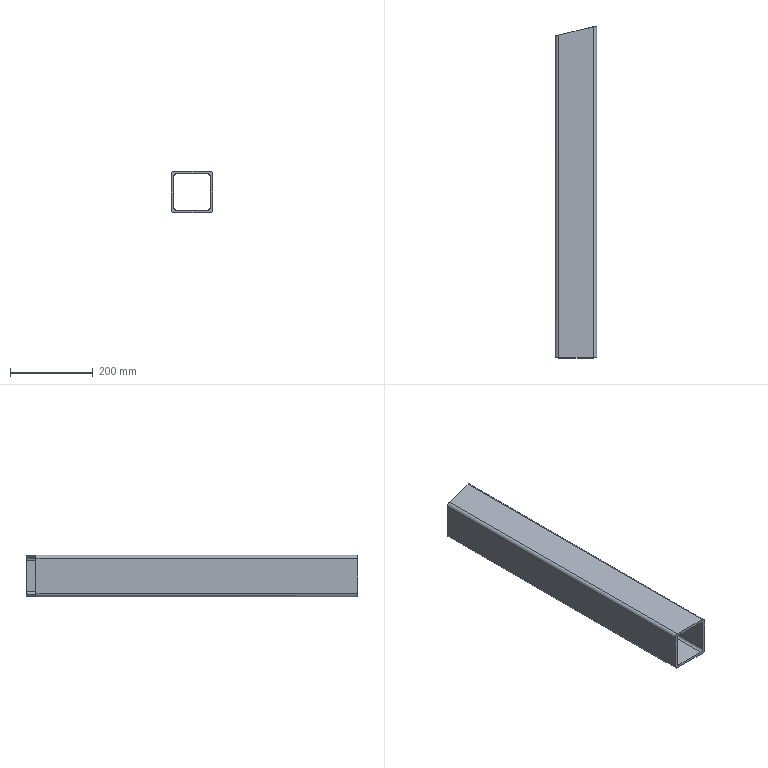Part | SolidWorks | features Extrusion 1, ICE 1 | 1 solid | 18 faces | box 100 x 800 x 100 mm | volume 1845556 mm3 | plane 10 | cylinder 8 | commonest cylinder face diameters 12.6 x4 15.75 x4
STEP:
#1=CARTESIAN_POINT('',(100.,-400.,-90.6));
#2=VERTEX_POINT('',#1);
#3=CARTESIAN_POINT('',(92.125,-400.,-98.475));
#4=VERTEX_POINT('',#3);
#5=CARTESIAN_POINT('',(92.125,-400.,-90.6));
#6=DIRECTION('',(0.,1.,0.));
#7=DIRECTION('',(0.,0.,1.));
#8=AXIS2_PLACEMENT_3D('',#5,#6,#7);
#9=CIRCLE('',#8,7.875);
#10=EDGE_CURVE('',#2,#4,#9,.T.);
#11=ORIENTED_EDGE('',*,*,#10,.F.);
#12=CARTESIAN_POINT('',(100.,-400.,-6.35));
#13=VERTEX_POINT('',#12);
#14=CARTESIAN_POINT('',(100.,-400.,-90.6));
#15=DIRECTION('',(0.,0.,-1.));
#16=VECTOR('',#15,1000.);
#17=LINE('',#14,#16);
#18=EDGE_CURVE('',#13,#2,#17,.T.);
#19=ORIENTED_EDGE('',*,*,#18,.F.);
#20=CARTESIAN_POINT('',(92.125,-400.,1.525));
#21=VERTEX_POINT('',#20);
#22=CARTESIAN_POINT('',(92.125,-400.,-6.35));
#23=DIRECTION('',(0.,1.,0.));
#24=DIRECTION('',(0.,0.,1.));
#25=AXIS2_PLACEMENT_3D('',#22,#23,#24);
#26=CIRCLE('',#25,7.875);
#27=EDGE_CURVE('',#21,#13,#26,.T.);
#28=ORIENTED_EDGE('',*,*,#27,.F.);
#29=CARTESIAN_POINT('',(7.875,-400.,1.525));
#30=VERTEX_POINT('',#29);
#31=CARTESIAN_POINT('',(7.875,-400.,1.525));
#32=DIRECTION('',(1.,0.,0.));
#33=VECTOR('',#32,1000.);
#34=LINE('',#31,#33);
#35=EDGE_CURVE('',#30,#21,#34,.T.);
#36=ORIENTED_EDGE('',*,*,#35,.F.);
#37=CARTESIAN_POINT('',(0.,-400.,-6.35));
#38=VERTEX_POINT('',#37);
#39=CARTESIAN_POINT('',(7.875,-400.,-6.35));
#40=DIRECTION('',(0.,1.,0.));
#41=DIRECTION('',(0.,0.,1.));
#42=AXIS2_PLACEMENT_3D('',#39,#40,#41);
#43=CIRCLE('',#42,7.875);
#44=EDGE_CURVE('',#38,#30,#43,.T.);
#45=ORIENTED_EDGE('',*,*,#44,.F.);
#46=CARTESIAN_POINT('',(0.,-400.,-90.6));
#47=VERTEX_POINT('',#46);
#48=CARTESIAN_POINT('',(0.,-400.,-6.35));
#49=DIRECTION('',(0.,0.,1.));
#50=VECTOR('',#49,1000.);
#51=LINE('',#48,#50);
#52=EDGE_CURVE('',#47,#38,#51,.T.);
#53=ORIENTED_EDGE('',*,*,#52,.F.);
#54=CARTESIAN_POINT('',(7.875,-400.,-98.475));
#55=VERTEX_POINT('',#54);
#56=CARTESIAN_POINT('',(7.875,-400.,-90.6));
#57=DIRECTION('',(0.,1.,0.));
#58=DIRECTION('',(0.,0.,1.));
#59=AXIS2_PLACEMENT_3D('',#56,#57,#58);
#60=CIRCLE('',#59,7.875);
#61=EDGE_CURVE('',#55,#47,#60,.T.);
#62=ORIENTED_EDGE('',*,*,#61,.F.);
#63=CARTESIAN_POINT('',(92.125,-400.,-98.475));
#64=DIRECTION('',(-1.,0.,0.));
#65=VECTOR('',#64,1000.);
#66=LINE('',#63,#65);
#67=EDGE_CURVE('',#4,#55,#66,.T.);
#68=ORIENTED_EDGE('',*,*,#67,.F.);
#69=EDGE_LOOP('',(#11,#19,#28,#36,#45,#53,#62,#68));
#70=FACE_OUTER_BOUND('',#69,.T.);
#71=CARTESIAN_POINT('',(12.6,-400.,-92.175));
#72=VERTEX_POINT('',#71);
#73=CARTESIAN_POINT('',(6.3,-400.,-85.875));
#74=VERTEX_POINT('',#73);
#75=CARTESIAN_POINT('',(12.6,-400.,-85.875));
#76=DIRECTION('',(0.,1.,0.));
#77=DIRECTION('',(0.,0.,1.));
#78=AXIS2_PLACEMENT_3D('',#75,#76,#77);
#79=CIRCLE('',#78,6.3);
#80=EDGE_CURVE('',#72,#74,#79,.T.);
#81=ORIENTED_EDGE('',*,*,#80,.T.);
#82=CARTESIAN_POINT('',(6.3,-400.,-11.075));
#83=VERTEX_POINT('',#82);
#84=CARTESIAN_POINT('',(6.3,-400.,-11.075));
#85=DIRECTION('',(0.,0.,1.));
#86=VECTOR('',#85,1000.);
#87=LINE('',#84,#86);
#88=EDGE_CURVE('',#74,#83,#87,.T.);
#89=ORIENTED_EDGE('',*,*,#88,.T.);
#90=CARTESIAN_POINT('',(12.6,-400.,-4.775));
#91=VERTEX_POINT('',#90);
#92=CARTESIAN_POINT('',(12.6,-400.,-11.075));
#93=DIRECTION('',(0.,1.,0.));
#94=DIRECTION('',(0.,0.,1.));
#95=AXIS2_PLACEMENT_3D('',#92,#93,#94);
#96=CIRCLE('',#95,6.3);
#97=EDGE_CURVE('',#83,#91,#96,.T.);
#98=ORIENTED_EDGE('',*,*,#97,.T.);
#99=CARTESIAN_POINT('',(87.4,-400.,-4.775));
#100=VERTEX_POINT('',#99);
#101=CARTESIAN_POINT('',(12.6,-400.,-4.775));
#102=DIRECTION('',(1.,0.,0.));
#103=VECTOR('',#102,1000.);
#104=LINE('',#101,#103);
#105=EDGE_CURVE('',#91,#100,#104,.T.);
#106=ORIENTED_EDGE('',*,*,#105,.T.);
#107=CARTESIAN_POINT('',(93.7,-400.,-11.075));
#108=VERTEX_POINT('',#107);
#109=CARTESIAN_POINT('',(87.4,-400.,-11.075));
#110=DIRECTION('',(0.,1.,0.));
#111=DIRECTION('',(0.,0.,1.));
#112=AXIS2_PLACEMENT_3D('',#109,#110,#111);
#113=CIRCLE('',#112,6.3);
#114=EDGE_CURVE('',#100,#108,#113,.T.);
#115=ORIENTED_EDGE('',*,*,#114,.T.);
#116=CARTESIAN_POINT('',(93.7,-400.,-85.875));
#117=VERTEX_POINT('',#116);
#118=CARTESIAN_POINT('',(93.7,-400.,-85.875));
#119=DIRECTION('',(0.,0.,-1.));
#120=VECTOR('',#119,1000.);
#121=LINE('',#118,#120);
#122=EDGE_CURVE('',#108,#117,#121,.T.);
#123=ORIENTED_EDGE('',*,*,#122,.T.);
#124=CARTESIAN_POINT('',(87.4,-400.,-92.175));
#125=VERTEX_POINT('',#124);
#126=CARTESIAN_POINT('',(87.4,-400.,-85.875));
#127=DIRECTION('',(0.,1.,0.));
#128=DIRECTION('',(0.,0.,1.));
#129=AXIS2_PLACEMENT_3D('',#126,#127,#128);
#130=CIRCLE('',#129,6.3);
#131=EDGE_CURVE('',#117,#125,#130,.T.);
#132=ORIENTED_EDGE('',*,*,#131,.T.);
#133=CARTESIAN_POINT('',(87.4,-400.,-92.175));
#134=DIRECTION('',(-1.,0.,0.));
#135=VECTOR('',#134,1000.);
#136=LINE('',#133,#135);
#137=EDGE_CURVE('',#125,#72,#136,.T.);
#138=ORIENTED_EDGE('',*,*,#137,.T.);
#139=EDGE_LOOP('',(#81,#89,#98,#106,#115,#123,#132,#138));
#140=FACE_BOUND('',#139,.T.);
#141=CARTESIAN_POINT('',(92.125,-400.,-90.6));
#142=DIRECTION('',(0.,1.,0.));
#143=DIRECTION('',(0.,0.,1.));
#144=AXIS2_PLACEMENT_3D('',#141,#142,#143);
#145=PLANE('',#144);
#146=ADVANCED_FACE('',(#70,#140),#145,.F.);
#147=CARTESIAN_POINT('',(92.125,398.11,-98.475));
#148=VERTEX_POINT('',#147);
#149=CARTESIAN_POINT('',(92.125,400.,-98.475));
#150=DIRECTION('',(0.,-1.,0.));
#151=VECTOR('',#150,1000.);
#152=LINE('',#149,#151);
#153=EDGE_CURVE('',#148,#4,#152,.T.);
#154=ORIENTED_EDGE('',*,*,#153,.F.);
#155=CARTESIAN_POINT('',(100.,400.,-90.6));
#156=VERTEX_POINT('',#155);
#157=CARTESIAN_POINT('',(100.,400.,-90.6));
#158=CARTESIAN_POINT('',(100.,400.,-95.213));
#159=CARTESIAN_POINT('',(96.738,399.217,-98.475));
#160=CARTESIAN_POINT('',(92.125,398.11,-98.475));
#161=(BOUNDED_CURVE()B_SPLINE_CURVE(3,(#157,#158,#159,#160),.UNSPECIFIED.,.F.,.F.)B_SPLINE_CURVE_WITH_KNOTS((4,4),(3.142,4.712),.UNSPECIFIED.)CURVE()GEOMETRIC_REPRESENTATION_ITEM()RATIONAL_B_SPLINE_CURVE((1.,0.8047,0.8047,1.))REPRESENTATION_ITEM(''));
#162=EDGE_CURVE('',#156,#148,#161,.T.);
#163=ORIENTED_EDGE('',*,*,#162,.F.);
#164=CARTESIAN_POINT('',(100.,400.,-90.6));
#165=DIRECTION('',(0.,-1.,0.));
#166=VECTOR('',#165,1000.);
#167=LINE('',#164,#166);
#168=EDGE_CURVE('',#156,#2,#167,.T.);
#169=ORIENTED_EDGE('',*,*,#168,.T.);
#170=ORIENTED_EDGE('',*,*,#10,.T.);
#171=EDGE_LOOP('',(#154,#163,#169,#170));
#172=FACE_OUTER_BOUND('',#171,.T.);
#173=CARTESIAN_POINT('',(92.125,400.,-90.6));
#174=DIRECTION('',(0.,-1.,0.));
#175=DIRECTION('',(0.,0.,-1.));
#176=AXIS2_PLACEMENT_3D('',#173,#174,#175);
#177=CYLINDRICAL_SURFACE('',#176,7.875);
#178=ADVANCED_FACE('',(#172),#177,.T.);
#179=CARTESIAN_POINT('',(7.875,377.89,-98.475));
#180=VERTEX_POINT('',#179);
#181=CARTESIAN_POINT('',(7.875,400.,-98.475));
#182=DIRECTION('',(0.,-1.,0.));
#183=VECTOR('',#182,1000.);
#184=LINE('',#181,#183);
#185=EDGE_CURVE('',#180,#55,#184,.T.);
#186=ORIENTED_EDGE('',*,*,#185,.F.);
#187=CARTESIAN_POINT('',(100.,400.,-98.475));
#188=DIRECTION('',(-0.9724,-0.2334,0.));
#189=VECTOR('',#188,1000.);
#190=LINE('',#187,#189);
#191=EDGE_CURVE('',#148,#180,#190,.T.);
#192=ORIENTED_EDGE('',*,*,#191,.F.);
#193=ORIENTED_EDGE('',*,*,#153,.T.);
#194=ORIENTED_EDGE('',*,*,#67,.T.);
#195=EDGE_LOOP('',(#186,#192,#193,#194));
#196=FACE_OUTER_BOUND('',#195,.T.);
#197=CARTESIAN_POINT('',(92.125,400.,-98.475));
#198=DIRECTION('',(0.,0.,1.));
#199=DIRECTION('',(1.,0.,0.));
#200=AXIS2_PLACEMENT_3D('',#197,#198,#199);
#201=PLANE('',#200);
#202=ADVANCED_FACE('',(#196),#201,.F.);
#203=CARTESIAN_POINT('',(0.,376.,-90.6));
#204=VERTEX_POINT('',#203);
#205=CARTESIAN_POINT('',(0.,400.,-90.6));
#206=DIRECTION('',(0.,-1.,0.));
#207=VECTOR('',#206,1000.);
#208=LINE('',#205,#207);
#209=EDGE_CURVE('',#204,#47,#208,.T.);
#210=ORIENTED_EDGE('',*,*,#209,.F.);
#211=CARTESIAN_POINT('',(7.875,377.89,-98.475));
#212=CARTESIAN_POINT('',(3.262,376.783,-98.475));
#213=CARTESIAN_POINT('',(0.,376.,-95.213));
#214=CARTESIAN_POINT('',(0.,376.,-90.6));
#215=(BOUNDED_CURVE()B_SPLINE_CURVE(3,(#211,#212,#213,#214),.UNSPECIFIED.,.F.,.T.)B_SPLINE_CURVE_WITH_KNOTS((4,4),(4.712,6.283),.UNSPECIFIED.)CURVE()GEOMETRIC_REPRESENTATION_ITEM()RATIONAL_B_SPLINE_CURVE((1.,0.8047,0.8047,1.))REPRESENTATION_ITEM(''));
#216=EDGE_CURVE('',#180,#204,#215,.T.);
#217=ORIENTED_EDGE('',*,*,#216,.F.);
#218=ORIENTED_EDGE('',*,*,#185,.T.);
#219=ORIENTED_EDGE('',*,*,#61,.T.);
#220=EDGE_LOOP('',(#210,#217,#218,#219));
#221=FACE_OUTER_BOUND('',#220,.T.);
#222=CARTESIAN_POINT('',(7.875,400.,-90.6));
#223=DIRECTION('',(0.,-1.,0.));
#224=DIRECTION('',(0.,0.,-1.));
#225=AXIS2_PLACEMENT_3D('',#222,#223,#224);
#226=CYLINDRICAL_SURFACE('',#225,7.875);
#227=ADVANCED_FACE('',(#221),#226,.T.);
#228=CARTESIAN_POINT('',(0.,376.,-6.35));
#229=VERTEX_POINT('',#228);
#230=CARTESIAN_POINT('',(0.,400.,-6.35));
#231=DIRECTION('',(0.,-1.,0.));
#232=VECTOR('',#231,1000.);
#233=LINE('',#230,#232);
#234=EDGE_CURVE('',#229,#38,#233,.T.);
#235=ORIENTED_EDGE('',*,*,#234,.F.);
#236=CARTESIAN_POINT('',(0.,376.,-98.476));
#237=DIRECTION('',(0.,0.,1.));
#238=VECTOR('',#237,1000.);
#239=LINE('',#236,#238);
#240=EDGE_CURVE('',#204,#229,#239,.T.);
#241=ORIENTED_EDGE('',*,*,#240,.F.);
#242=ORIENTED_EDGE('',*,*,#209,.T.);
#243=ORIENTED_EDGE('',*,*,#52,.T.);
#244=EDGE_LOOP('',(#235,#241,#242,#243));
#245=FACE_OUTER_BOUND('',#244,.T.);
#246=CARTESIAN_POINT('',(0.,400.,-6.35));
#247=DIRECTION('',(1.,0.,0.));
#248=DIRECTION('',(0.,0.,-1.));
#249=AXIS2_PLACEMENT_3D('',#246,#247,#248);
#250=PLANE('',#249);
#251=ADVANCED_FACE('',(#245),#250,.F.);
#252=CARTESIAN_POINT('',(7.875,377.89,1.525));
#253=VERTEX_POINT('',#252);
#254=CARTESIAN_POINT('',(7.875,400.,1.525));
#255=DIRECTION('',(0.,-1.,0.));
#256=VECTOR('',#255,1000.);
#257=LINE('',#254,#256);
#258=EDGE_CURVE('',#253,#30,#257,.T.);
#259=ORIENTED_EDGE('',*,*,#258,.F.);
#260=CARTESIAN_POINT('',(0.,376.,-6.35));
#261=CARTESIAN_POINT('',(0.,376.,-1.737));
#262=CARTESIAN_POINT('',(3.262,376.783,1.525));
#263=CARTESIAN_POINT('',(7.875,377.89,1.525));
#264=(BOUNDED_CURVE()B_SPLINE_CURVE(3,(#260,#261,#262,#263),.UNSPECIFIED.,.F.,.T.)B_SPLINE_CURVE_WITH_KNOTS((4,4),(0.,1.571),.UNSPECIFIED.)CURVE()GEOMETRIC_REPRESENTATION_ITEM()RATIONAL_B_SPLINE_CURVE((1.,0.8047,0.8047,1.))REPRESENTATION_ITEM(''));
#265=EDGE_CURVE('',#229,#253,#264,.T.);
#266=ORIENTED_EDGE('',*,*,#265,.F.);
#267=ORIENTED_EDGE('',*,*,#234,.T.);
#268=ORIENTED_EDGE('',*,*,#44,.T.);
#269=EDGE_LOOP('',(#259,#266,#267,#268));
#270=FACE_OUTER_BOUND('',#269,.T.);
#271=CARTESIAN_POINT('',(7.875,400.,-6.35));
#272=DIRECTION('',(0.,-1.,0.));
#273=DIRECTION('',(0.,0.,-1.));
#274=AXIS2_PLACEMENT_3D('',#271,#272,#273);
#275=CYLINDRICAL_SURFACE('',#274,7.875);
#276=ADVANCED_FACE('',(#270),#275,.T.);
#277=CARTESIAN_POINT('',(92.125,398.11,1.525));
#278=VERTEX_POINT('',#277);
#279=CARTESIAN_POINT('',(92.125,400.,1.525));
#280=DIRECTION('',(0.,-1.,0.));
#281=VECTOR('',#280,1000.);
#282=LINE('',#279,#281);
#283=EDGE_CURVE('',#278,#21,#282,.T.);
#284=ORIENTED_EDGE('',*,*,#283,.F.);
#285=CARTESIAN_POINT('',(100.,400.,1.525));
#286=DIRECTION('',(0.9724,0.2334,0.));
#287=VECTOR('',#286,1000.);
#288=LINE('',#285,#287);
#289=EDGE_CURVE('',#253,#278,#288,.T.);
#290=ORIENTED_EDGE('',*,*,#289,.F.);
#291=ORIENTED_EDGE('',*,*,#258,.T.);
#292=ORIENTED_EDGE('',*,*,#35,.T.);
#293=EDGE_LOOP('',(#284,#290,#291,#292));
#294=FACE_OUTER_BOUND('',#293,.T.);
#295=CARTESIAN_POINT('',(7.875,400.,1.525));
#296=DIRECTION('',(0.,0.,-1.));
#297=DIRECTION('',(-1.,0.,0.));
#298=AXIS2_PLACEMENT_3D('',#295,#296,#297);
#299=PLANE('',#298);
#300=ADVANCED_FACE('',(#294),#299,.F.);
#301=CARTESIAN_POINT('',(100.,400.,-6.35));
#302=VERTEX_POINT('',#301);
#303=CARTESIAN_POINT('',(100.,400.,-6.35));
#304=DIRECTION('',(0.,-1.,0.));
#305=VECTOR('',#304,1000.);
#306=LINE('',#303,#305);
#307=EDGE_CURVE('',#302,#13,#306,.T.);
#308=ORIENTED_EDGE('',*,*,#307,.F.);
#309=CARTESIAN_POINT('',(92.125,398.11,1.525));
#310=CARTESIAN_POINT('',(96.738,399.217,1.525));
#311=CARTESIAN_POINT('',(100.,400.,-1.737));
#312=CARTESIAN_POINT('',(100.,400.,-6.35));
#313=(BOUNDED_CURVE()B_SPLINE_CURVE(3,(#309,#310,#311,#312),.UNSPECIFIED.,.F.,.F.)B_SPLINE_CURVE_WITH_KNOTS((4,4),(1.571,3.142),.UNSPECIFIED.)CURVE()GEOMETRIC_REPRESENTATION_ITEM()RATIONAL_B_SPLINE_CURVE((1.,0.8047,0.8047,1.))REPRESENTATION_ITEM(''));
#314=EDGE_CURVE('',#278,#302,#313,.T.);
#315=ORIENTED_EDGE('',*,*,#314,.F.);
#316=ORIENTED_EDGE('',*,*,#283,.T.);
#317=ORIENTED_EDGE('',*,*,#27,.T.);
#318=EDGE_LOOP('',(#308,#315,#316,#317));
#319=FACE_OUTER_BOUND('',#318,.T.);
#320=CARTESIAN_POINT('',(92.125,400.,-6.35));
#321=DIRECTION('',(0.,-1.,0.));
#322=DIRECTION('',(0.,0.,-1.));
#323=AXIS2_PLACEMENT_3D('',#320,#321,#322);
#324=CYLINDRICAL_SURFACE('',#323,7.875);
#325=ADVANCED_FACE('',(#319),#324,.T.);
#326=ORIENTED_EDGE('',*,*,#18,.T.);
#327=ORIENTED_EDGE('',*,*,#168,.F.);
#328=CARTESIAN_POINT('',(100.,400.,-90.6));
#329=DIRECTION('',(0.,0.,-1.));
#330=VECTOR('',#329,1000.);
#331=LINE('',#328,#330);
#332=EDGE_CURVE('',#302,#156,#331,.T.);
#333=ORIENTED_EDGE('',*,*,#332,.F.);
#334=ORIENTED_EDGE('',*,*,#307,.T.);
#335=EDGE_LOOP('',(#326,#327,#333,#334));
#336=FACE_OUTER_BOUND('',#335,.T.);
#337=CARTESIAN_POINT('',(100.,400.,-90.6));
#338=DIRECTION('',(-1.,0.,0.));
#339=DIRECTION('',(0.,0.,1.));
#340=AXIS2_PLACEMENT_3D('',#337,#338,#339);
#341=PLANE('',#340);
#342=ADVANCED_FACE('',(#336),#341,.F.);
#343=CARTESIAN_POINT('',(12.6,379.024,-92.175));
#344=VERTEX_POINT('',#343);
#345=CARTESIAN_POINT('',(6.3,377.512,-85.875));
#346=VERTEX_POINT('',#345);
#347=CARTESIAN_POINT('',(12.6,379.024,-92.175));
#348=CARTESIAN_POINT('',(8.91,378.138,-92.175));
#349=CARTESIAN_POINT('',(6.3,377.512,-89.565));
#350=CARTESIAN_POINT('',(6.3,377.512,-85.875));
#351=(BOUNDED_CURVE()B_SPLINE_CURVE(3,(#347,#348,#349,#350),.UNSPECIFIED.,.F.,.T.)B_SPLINE_CURVE_WITH_KNOTS((4,4),(4.712,6.283),.UNSPECIFIED.)CURVE()GEOMETRIC_REPRESENTATION_ITEM()RATIONAL_B_SPLINE_CURVE((1.,0.8047,0.8047,1.))REPRESENTATION_ITEM(''));
#352=EDGE_CURVE('',#344,#346,#351,.T.);
#353=ORIENTED_EDGE('',*,*,#352,.T.);
#354=CARTESIAN_POINT('',(6.3,400.,-85.875));
#355=DIRECTION('',(0.,-1.,0.));
#356=VECTOR('',#355,1000.);
#357=LINE('',#354,#356);
#358=EDGE_CURVE('',#346,#74,#357,.T.);
#359=ORIENTED_EDGE('',*,*,#358,.T.);
#360=ORIENTED_EDGE('',*,*,#80,.F.);
#361=CARTESIAN_POINT('',(12.6,400.,-92.175));
#362=DIRECTION('',(0.,-1.,0.));
#363=VECTOR('',#362,1000.);
#364=LINE('',#361,#363);
#365=EDGE_CURVE('',#344,#72,#364,.T.);
#366=ORIENTED_EDGE('',*,*,#365,.F.);
#367=EDGE_LOOP('',(#353,#359,#360,#366));
#368=FACE_OUTER_BOUND('',#367,.T.);
#369=CARTESIAN_POINT('',(12.6,400.,-85.875));
#370=DIRECTION('',(0.,-1.,0.));
#371=DIRECTION('',(0.,0.,-1.));
#372=AXIS2_PLACEMENT_3D('',#369,#370,#371);
#373=CYLINDRICAL_SURFACE('',#372,6.3);
#374=ADVANCED_FACE('',(#368),#373,.F.);
#375=CARTESIAN_POINT('',(6.3,377.512,-11.075));
#376=VERTEX_POINT('',#375);
#377=CARTESIAN_POINT('',(6.3,377.512,-98.476));
#378=DIRECTION('',(0.,0.,1.));
#379=VECTOR('',#378,1000.);
#380=LINE('',#377,#379);
#381=EDGE_CURVE('',#346,#376,#380,.T.);
#382=ORIENTED_EDGE('',*,*,#381,.T.);
#383=CARTESIAN_POINT('',(6.3,400.,-11.075));
#384=DIRECTION('',(0.,-1.,0.));
#385=VECTOR('',#384,1000.);
#386=LINE('',#383,#385);
#387=EDGE_CURVE('',#376,#83,#386,.T.);
#388=ORIENTED_EDGE('',*,*,#387,.T.);
#389=ORIENTED_EDGE('',*,*,#88,.F.);
#390=ORIENTED_EDGE('',*,*,#358,.F.);
#391=EDGE_LOOP('',(#382,#388,#389,#390));
#392=FACE_OUTER_BOUND('',#391,.T.);
#393=CARTESIAN_POINT('',(6.3,400.,-11.075));
#394=DIRECTION('',(1.,0.,0.));
#395=DIRECTION('',(0.,0.,-1.));
#396=AXIS2_PLACEMENT_3D('',#393,#394,#395);
#397=PLANE('',#396);
#398=ADVANCED_FACE('',(#392),#397,.T.);
#399=CARTESIAN_POINT('',(12.6,379.024,-4.775));
#400=VERTEX_POINT('',#399);
#401=CARTESIAN_POINT('',(6.3,377.512,-11.075));
#402=CARTESIAN_POINT('',(6.3,377.512,-7.385));
#403=CARTESIAN_POINT('',(8.91,378.138,-4.775));
#404=CARTESIAN_POINT('',(12.6,379.024,-4.775));
#405=(BOUNDED_CURVE()B_SPLINE_CURVE(3,(#401,#402,#403,#404),.UNSPECIFIED.,.F.,.T.)B_SPLINE_CURVE_WITH_KNOTS((4,4),(0.,1.571),.UNSPECIFIED.)CURVE()GEOMETRIC_REPRESENTATION_ITEM()RATIONAL_B_SPLINE_CURVE((1.,0.8047,0.8047,1.))REPRESENTATION_ITEM(''));
#406=EDGE_CURVE('',#376,#400,#405,.T.);
#407=ORIENTED_EDGE('',*,*,#406,.T.);
#408=CARTESIAN_POINT('',(12.6,400.,-4.775));
#409=DIRECTION('',(0.,-1.,0.));
#410=VECTOR('',#409,1000.);
#411=LINE('',#408,#410);
#412=EDGE_CURVE('',#400,#91,#411,.T.);
#413=ORIENTED_EDGE('',*,*,#412,.T.);
#414=ORIENTED_EDGE('',*,*,#97,.F.);
#415=ORIENTED_EDGE('',*,*,#387,.F.);
#416=EDGE_LOOP('',(#407,#413,#414,#415));
#417=FACE_OUTER_BOUND('',#416,.T.);
#418=CARTESIAN_POINT('',(12.6,400.,-11.075));
#419=DIRECTION('',(0.,-1.,0.));
#420=DIRECTION('',(0.,0.,-1.));
#421=AXIS2_PLACEMENT_3D('',#418,#419,#420);
#422=CYLINDRICAL_SURFACE('',#421,6.3);
#423=ADVANCED_FACE('',(#417),#422,.F.);
#424=CARTESIAN_POINT('',(87.4,396.976,-4.775));
#425=VERTEX_POINT('',#424);
#426=CARTESIAN_POINT('',(100.,400.,-4.775));
#427=DIRECTION('',(0.9724,0.2334,0.));
#428=VECTOR('',#427,1000.);
#429=LINE('',#426,#428);
#430=EDGE_CURVE('',#400,#425,#429,.T.);
#431=ORIENTED_EDGE('',*,*,#430,.T.);
#432=CARTESIAN_POINT('',(87.4,400.,-4.775));
#433=DIRECTION('',(0.,-1.,0.));
#434=VECTOR('',#433,1000.);
#435=LINE('',#432,#434);
#436=EDGE_CURVE('',#425,#100,#435,.T.);
#437=ORIENTED_EDGE('',*,*,#436,.T.);
#438=ORIENTED_EDGE('',*,*,#105,.F.);
#439=ORIENTED_EDGE('',*,*,#412,.F.);
#440=EDGE_LOOP('',(#431,#437,#438,#439));
#441=FACE_OUTER_BOUND('',#440,.T.);
#442=CARTESIAN_POINT('',(12.6,400.,-4.775));
#443=DIRECTION('',(0.,0.,-1.));
#444=DIRECTION('',(-1.,0.,0.));
#445=AXIS2_PLACEMENT_3D('',#442,#443,#444);
#446=PLANE('',#445);
#447=ADVANCED_FACE('',(#441),#446,.T.);
#448=CARTESIAN_POINT('',(93.7,398.488,-11.075));
#449=VERTEX_POINT('',#448);
#450=CARTESIAN_POINT('',(87.4,396.976,-4.775));
#451=CARTESIAN_POINT('',(91.09,397.862,-4.775));
#452=CARTESIAN_POINT('',(93.7,398.488,-7.385));
#453=CARTESIAN_POINT('',(93.7,398.488,-11.075));
#454=(BOUNDED_CURVE()B_SPLINE_CURVE(3,(#450,#451,#452,#453),.UNSPECIFIED.,.F.,.T.)B_SPLINE_CURVE_WITH_KNOTS((4,4),(1.571,3.142),.UNSPECIFIED.)CURVE()GEOMETRIC_REPRESENTATION_ITEM()RATIONAL_B_SPLINE_CURVE((1.,0.8047,0.8047,1.))REPRESENTATION_ITEM(''));
#455=EDGE_CURVE('',#425,#449,#454,.T.);
#456=ORIENTED_EDGE('',*,*,#455,.T.);
#457=CARTESIAN_POINT('',(93.7,400.,-11.075));
#458=DIRECTION('',(0.,-1.,0.));
#459=VECTOR('',#458,1000.);
#460=LINE('',#457,#459);
#461=EDGE_CURVE('',#449,#108,#460,.T.);
#462=ORIENTED_EDGE('',*,*,#461,.T.);
#463=ORIENTED_EDGE('',*,*,#114,.F.);
#464=ORIENTED_EDGE('',*,*,#436,.F.);
#465=EDGE_LOOP('',(#456,#462,#463,#464));
#466=FACE_OUTER_BOUND('',#465,.T.);
#467=CARTESIAN_POINT('',(87.4,400.,-11.075));
#468=DIRECTION('',(0.,-1.,0.));
#469=DIRECTION('',(0.,0.,-1.));
#470=AXIS2_PLACEMENT_3D('',#467,#468,#469);
#471=CYLINDRICAL_SURFACE('',#470,6.3);
#472=ADVANCED_FACE('',(#466),#471,.F.);
#473=CARTESIAN_POINT('',(93.7,398.488,-85.875));
#474=VERTEX_POINT('',#473);
#475=CARTESIAN_POINT('',(93.7,398.488,-98.476));
#476=DIRECTION('',(0.,0.,-1.));
#477=VECTOR('',#476,1000.);
#478=LINE('',#475,#477);
#479=EDGE_CURVE('',#449,#474,#478,.T.);
#480=ORIENTED_EDGE('',*,*,#479,.T.);
#481=CARTESIAN_POINT('',(93.7,400.,-85.875));
#482=DIRECTION('',(0.,-1.,0.));
#483=VECTOR('',#482,1000.);
#484=LINE('',#481,#483);
#485=EDGE_CURVE('',#474,#117,#484,.T.);
#486=ORIENTED_EDGE('',*,*,#485,.T.);
#487=ORIENTED_EDGE('',*,*,#122,.F.);
#488=ORIENTED_EDGE('',*,*,#461,.F.);
#489=EDGE_LOOP('',(#480,#486,#487,#488));
#490=FACE_OUTER_BOUND('',#489,.T.);
#491=CARTESIAN_POINT('',(93.7,400.,-85.875));
#492=DIRECTION('',(-1.,0.,0.));
#493=DIRECTION('',(0.,0.,1.));
#494=AXIS2_PLACEMENT_3D('',#491,#492,#493);
#495=PLANE('',#494);
#496=ADVANCED_FACE('',(#490),#495,.T.);
#497=CARTESIAN_POINT('',(87.4,396.976,-92.175));
#498=VERTEX_POINT('',#497);
#499=CARTESIAN_POINT('',(93.7,398.488,-85.875));
#500=CARTESIAN_POINT('',(93.7,398.488,-89.565));
#501=CARTESIAN_POINT('',(91.09,397.862,-92.175));
#502=CARTESIAN_POINT('',(87.4,396.976,-92.175));
#503=(BOUNDED_CURVE()B_SPLINE_CURVE(3,(#499,#500,#501,#502),.UNSPECIFIED.,.F.,.T.)B_SPLINE_CURVE_WITH_KNOTS((4,4),(3.142,4.712),.UNSPECIFIED.)CURVE()GEOMETRIC_REPRESENTATION_ITEM()RATIONAL_B_SPLINE_CURVE((1.,0.8047,0.8047,1.))REPRESENTATION_ITEM(''));
#504=EDGE_CURVE('',#474,#498,#503,.T.);
#505=ORIENTED_EDGE('',*,*,#504,.T.);
#506=CARTESIAN_POINT('',(87.4,400.,-92.175));
#507=DIRECTION('',(0.,-1.,0.));
#508=VECTOR('',#507,1000.);
#509=LINE('',#506,#508);
#510=EDGE_CURVE('',#498,#125,#509,.T.);
#511=ORIENTED_EDGE('',*,*,#510,.T.);
#512=ORIENTED_EDGE('',*,*,#131,.F.);
#513=ORIENTED_EDGE('',*,*,#485,.F.);
#514=EDGE_LOOP('',(#505,#511,#512,#513));
#515=FACE_OUTER_BOUND('',#514,.T.);
#516=CARTESIAN_POINT('',(87.4,400.,-85.875));
#517=DIRECTION('',(0.,-1.,0.));
#518=DIRECTION('',(0.,0.,-1.));
#519=AXIS2_PLACEMENT_3D('',#516,#517,#518);
#520=CYLINDRICAL_SURFACE('',#519,6.3);
#521=ADVANCED_FACE('',(#515),#520,.F.);
#522=CARTESIAN_POINT('',(100.,400.,-92.175));
#523=DIRECTION('',(-0.9724,-0.2334,0.));
#524=VECTOR('',#523,1000.);
#525=LINE('',#522,#524);
#526=EDGE_CURVE('',#498,#344,#525,.T.);
#527=ORIENTED_EDGE('',*,*,#526,.T.);
#528=ORIENTED_EDGE('',*,*,#365,.T.);
#529=ORIENTED_EDGE('',*,*,#137,.F.);
#530=ORIENTED_EDGE('',*,*,#510,.F.);
#531=EDGE_LOOP('',(#527,#528,#529,#530));
#532=FACE_OUTER_BOUND('',#531,.T.);
#533=CARTESIAN_POINT('',(87.4,400.,-92.175));
#534=DIRECTION('',(0.,0.,1.));
#535=DIRECTION('',(1.,0.,0.));
#536=AXIS2_PLACEMENT_3D('',#533,#534,#535);
#537=PLANE('',#536);
#538=ADVANCED_FACE('',(#532),#537,.T.);
#539=ORIENTED_EDGE('',*,*,#526,.F.);
#540=ORIENTED_EDGE('',*,*,#504,.F.);
#541=ORIENTED_EDGE('',*,*,#479,.F.);
#542=ORIENTED_EDGE('',*,*,#455,.F.);
#543=ORIENTED_EDGE('',*,*,#430,.F.);
#544=ORIENTED_EDGE('',*,*,#406,.F.);
#545=ORIENTED_EDGE('',*,*,#381,.F.);
#546=ORIENTED_EDGE('',*,*,#352,.F.);
#547=EDGE_LOOP('',(#539,#540,#541,#542,#543,#544,#545,#546));
#548=FACE_BOUND('',#547,.T.);
#549=ORIENTED_EDGE('',*,*,#162,.T.);
#550=ORIENTED_EDGE('',*,*,#191,.T.);
#551=ORIENTED_EDGE('',*,*,#216,.T.);
#552=ORIENTED_EDGE('',*,*,#240,.T.);
#553=ORIENTED_EDGE('',*,*,#265,.T.);
#554=ORIENTED_EDGE('',*,*,#289,.T.);
#555=ORIENTED_EDGE('',*,*,#314,.T.);
#556=ORIENTED_EDGE('',*,*,#332,.T.);
#557=EDGE_LOOP('',(#549,#550,#551,#552,#553,#554,#555,#556));
#558=FACE_OUTER_BOUND('',#557,.T.);
#559=CARTESIAN_POINT('',(100.,400.,-98.476));
#560=DIRECTION('',(0.2334,-0.9724,0.));
#561=DIRECTION('',(0.9724,0.2334,0.));
#562=AXIS2_PLACEMENT_3D('',#559,#560,#561);
#563=PLANE('',#562);
#564=ADVANCED_FACE('',(#548,#558),#563,.F.);
#565=CLOSED_SHELL('',(#146,#178,#202,#227,#251,#276,#300,#325,#342,#374,#398,#423,#447,#472,#496,#521,#538,#564));
#566=MANIFOLD_SOLID_BREP('',#565);
#567=CARTESIAN_POINT('',(0.,0.,0.));
#568=DIRECTION('',(0.,0.,1.));
#569=DIRECTION('',(1.,0.,0.));
#570=AXIS2_PLACEMENT_3D('',#567,#568,#569);
#571=(LENGTH_UNIT()NAMED_UNIT(*)SI_UNIT(.MILLI.,.METRE.));
#572=UNCERTAINTY_MEASURE_WITH_UNIT(LENGTH_MEASURE(0.00001),#571,'','');
#573=(NAMED_UNIT(*)PLANE_ANGLE_UNIT()SI_UNIT($,.RADIAN.));
#574=(NAMED_UNIT(*)SI_UNIT($,.STERADIAN.)SOLID_ANGLE_UNIT());
#575=(GEOMETRIC_REPRESENTATION_CONTEXT(3)GLOBAL_UNCERTAINTY_ASSIGNED_CONTEXT((#572))GLOBAL_UNIT_ASSIGNED_CONTEXT((#571,#573,#574))REPRESENTATION_CONTEXT('',''));
#576=ADVANCED_BREP_SHAPE_REPRESENTATION('',(#566,#570),#575);